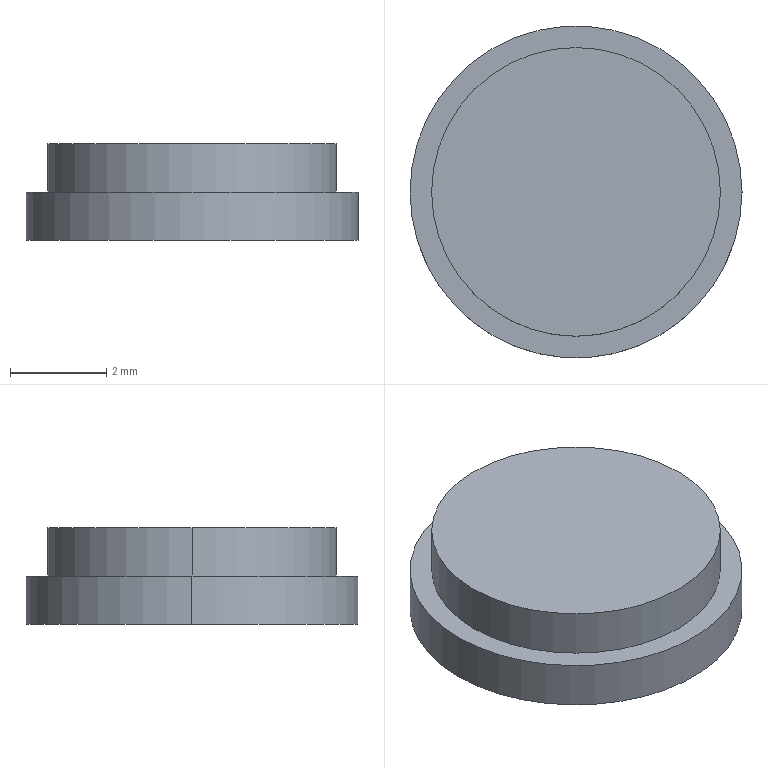Part | SolidWorks | features Extrusion 1, ICE 1 | 1 solid | 7 faces | box 6.9 x 6.9 x 2 mm | volume 65.667 mm3 | cylinder 4 | plane 3 | commonest cylinder face diameters 6 x2 6.9 x2
STEP:
#1=CARTESIAN_POINT('',(3.45,0.,-1.));
#2=VERTEX_POINT('',#1);
#3=CARTESIAN_POINT('',(-3.45,0.,-1.));
#4=VERTEX_POINT('',#3);
#5=CARTESIAN_POINT('',(0.,0.,-1.));
#6=DIRECTION('',(0.,0.,1.));
#7=DIRECTION('',(1.,0.,0.));
#8=AXIS2_PLACEMENT_3D('',#5,#6,#7);
#9=CIRCLE('',#8,3.45);
#10=EDGE_CURVE('',#2,#4,#9,.T.);
#11=ORIENTED_EDGE('',*,*,#10,.T.);
#12=CARTESIAN_POINT('',(-3.45,0.,0.));
#13=VERTEX_POINT('',#12);
#14=CARTESIAN_POINT('',(-3.45,0.,-1.));
#15=DIRECTION('',(0.,0.,1.));
#16=VECTOR('',#15,1000.);
#17=LINE('',#14,#16);
#18=EDGE_CURVE('',#4,#13,#17,.T.);
#19=ORIENTED_EDGE('',*,*,#18,.T.);
#20=CARTESIAN_POINT('',(3.45,0.,0.));
#21=VERTEX_POINT('',#20);
#22=CARTESIAN_POINT('',(0.,0.,0.));
#23=DIRECTION('',(0.,0.,1.));
#24=DIRECTION('',(1.,0.,0.));
#25=AXIS2_PLACEMENT_3D('',#22,#23,#24);
#26=CIRCLE('',#25,3.45);
#27=EDGE_CURVE('',#21,#13,#26,.T.);
#28=ORIENTED_EDGE('',*,*,#27,.F.);
#29=CARTESIAN_POINT('',(3.45,0.,-1.));
#30=DIRECTION('',(0.,0.,1.));
#31=VECTOR('',#30,1000.);
#32=LINE('',#29,#31);
#33=EDGE_CURVE('',#2,#21,#32,.T.);
#34=ORIENTED_EDGE('',*,*,#33,.F.);
#35=EDGE_LOOP('',(#11,#19,#28,#34));
#36=FACE_OUTER_BOUND('',#35,.T.);
#37=CARTESIAN_POINT('',(0.,0.,-1.));
#38=DIRECTION('',(0.,0.,1.));
#39=DIRECTION('',(1.,0.,0.));
#40=AXIS2_PLACEMENT_3D('',#37,#38,#39);
#41=CYLINDRICAL_SURFACE('',#40,3.45);
#42=ADVANCED_FACE('',(#36),#41,.T.);
#43=CARTESIAN_POINT('',(3.,0.,1.));
#44=VERTEX_POINT('',#43);
#45=CARTESIAN_POINT('',(-3.,0.,1.));
#46=VERTEX_POINT('',#45);
#47=CARTESIAN_POINT('',(0.,0.,1.));
#48=DIRECTION('',(0.,0.,1.));
#49=DIRECTION('',(1.,0.,0.));
#50=AXIS2_PLACEMENT_3D('',#47,#48,#49);
#51=CIRCLE('',#50,3.);
#52=EDGE_CURVE('',#44,#46,#51,.T.);
#53=ORIENTED_EDGE('',*,*,#52,.F.);
#54=CARTESIAN_POINT('',(3.,0.,0.));
#55=VERTEX_POINT('',#54);
#56=CARTESIAN_POINT('',(3.,0.,1.));
#57=DIRECTION('',(0.,0.,-1.));
#58=VECTOR('',#57,1000.);
#59=LINE('',#56,#58);
#60=EDGE_CURVE('',#44,#55,#59,.T.);
#61=ORIENTED_EDGE('',*,*,#60,.T.);
#62=CARTESIAN_POINT('',(-3.,0.,0.));
#63=VERTEX_POINT('',#62);
#64=CARTESIAN_POINT('',(0.,0.,0.));
#65=DIRECTION('',(0.,0.,1.));
#66=DIRECTION('',(1.,0.,0.));
#67=AXIS2_PLACEMENT_3D('',#64,#65,#66);
#68=CIRCLE('',#67,3.);
#69=EDGE_CURVE('',#55,#63,#68,.T.);
#70=ORIENTED_EDGE('',*,*,#69,.T.);
#71=CARTESIAN_POINT('',(-3.,0.,1.));
#72=DIRECTION('',(0.,0.,-1.));
#73=VECTOR('',#72,1000.);
#74=LINE('',#71,#73);
#75=EDGE_CURVE('',#46,#63,#74,.T.);
#76=ORIENTED_EDGE('',*,*,#75,.F.);
#77=EDGE_LOOP('',(#53,#61,#70,#76));
#78=FACE_OUTER_BOUND('',#77,.T.);
#79=CARTESIAN_POINT('',(0.,0.,1.));
#80=DIRECTION('',(0.,0.,-1.));
#81=DIRECTION('',(-1.,0.,0.));
#82=AXIS2_PLACEMENT_3D('',#79,#80,#81);
#83=CYLINDRICAL_SURFACE('',#82,3.);
#84=ADVANCED_FACE('',(#78),#83,.T.);
#85=ORIENTED_EDGE('',*,*,#60,.F.);
#86=CARTESIAN_POINT('',(0.,0.,1.));
#87=DIRECTION('',(0.,0.,1.));
#88=DIRECTION('',(1.,0.,0.));
#89=AXIS2_PLACEMENT_3D('',#86,#87,#88);
#90=CIRCLE('',#89,3.);
#91=EDGE_CURVE('',#46,#44,#90,.T.);
#92=ORIENTED_EDGE('',*,*,#91,.F.);
#93=ORIENTED_EDGE('',*,*,#75,.T.);
#94=CARTESIAN_POINT('',(0.,0.,0.));
#95=DIRECTION('',(0.,0.,1.));
#96=DIRECTION('',(1.,0.,0.));
#97=AXIS2_PLACEMENT_3D('',#94,#95,#96);
#98=CIRCLE('',#97,3.);
#99=EDGE_CURVE('',#63,#55,#98,.T.);
#100=ORIENTED_EDGE('',*,*,#99,.T.);
#101=EDGE_LOOP('',(#85,#92,#93,#100));
#102=FACE_OUTER_BOUND('',#101,.T.);
#103=CARTESIAN_POINT('',(0.,0.,1.));
#104=DIRECTION('',(0.,0.,-1.));
#105=DIRECTION('',(-1.,0.,0.));
#106=AXIS2_PLACEMENT_3D('',#103,#104,#105);
#107=CYLINDRICAL_SURFACE('',#106,3.);
#108=ADVANCED_FACE('',(#102),#107,.T.);
#109=ORIENTED_EDGE('',*,*,#91,.T.);
#110=ORIENTED_EDGE('',*,*,#52,.T.);
#111=EDGE_LOOP('',(#109,#110));
#112=FACE_OUTER_BOUND('',#111,.T.);
#113=CARTESIAN_POINT('',(0.,0.,1.));
#114=DIRECTION('',(0.,0.,1.));
#115=DIRECTION('',(1.,0.,0.));
#116=AXIS2_PLACEMENT_3D('',#113,#114,#115);
#117=PLANE('',#116);
#118=ADVANCED_FACE('',(#112),#117,.T.);
#119=ORIENTED_EDGE('',*,*,#18,.F.);
#120=CARTESIAN_POINT('',(0.,0.,-1.));
#121=DIRECTION('',(0.,0.,1.));
#122=DIRECTION('',(1.,0.,0.));
#123=AXIS2_PLACEMENT_3D('',#120,#121,#122);
#124=CIRCLE('',#123,3.45);
#125=EDGE_CURVE('',#4,#2,#124,.T.);
#126=ORIENTED_EDGE('',*,*,#125,.T.);
#127=ORIENTED_EDGE('',*,*,#33,.T.);
#128=CARTESIAN_POINT('',(0.,0.,0.));
#129=DIRECTION('',(0.,0.,1.));
#130=DIRECTION('',(1.,0.,0.));
#131=AXIS2_PLACEMENT_3D('',#128,#129,#130);
#132=CIRCLE('',#131,3.45);
#133=EDGE_CURVE('',#13,#21,#132,.T.);
#134=ORIENTED_EDGE('',*,*,#133,.F.);
#135=EDGE_LOOP('',(#119,#126,#127,#134));
#136=FACE_OUTER_BOUND('',#135,.T.);
#137=CARTESIAN_POINT('',(0.,0.,-1.));
#138=DIRECTION('',(0.,0.,1.));
#139=DIRECTION('',(1.,0.,0.));
#140=AXIS2_PLACEMENT_3D('',#137,#138,#139);
#141=CYLINDRICAL_SURFACE('',#140,3.45);
#142=ADVANCED_FACE('',(#136),#141,.T.);
#143=ORIENTED_EDGE('',*,*,#10,.F.);
#144=ORIENTED_EDGE('',*,*,#125,.F.);
#145=EDGE_LOOP('',(#143,#144));
#146=FACE_OUTER_BOUND('',#145,.T.);
#147=CARTESIAN_POINT('',(0.,0.,-1.));
#148=DIRECTION('',(0.,0.,1.));
#149=DIRECTION('',(1.,0.,0.));
#150=AXIS2_PLACEMENT_3D('',#147,#148,#149);
#151=PLANE('',#150);
#152=ADVANCED_FACE('',(#146),#151,.F.);
#153=ORIENTED_EDGE('',*,*,#99,.F.);
#154=ORIENTED_EDGE('',*,*,#69,.F.);
#155=EDGE_LOOP('',(#153,#154));
#156=FACE_BOUND('',#155,.T.);
#157=ORIENTED_EDGE('',*,*,#27,.T.);
#158=ORIENTED_EDGE('',*,*,#133,.T.);
#159=EDGE_LOOP('',(#157,#158));
#160=FACE_OUTER_BOUND('',#159,.T.);
#161=CARTESIAN_POINT('',(0.,0.,0.));
#162=DIRECTION('',(0.,0.,1.));
#163=DIRECTION('',(1.,0.,0.));
#164=AXIS2_PLACEMENT_3D('',#161,#162,#163);
#165=PLANE('',#164);
#166=ADVANCED_FACE('',(#156,#160),#165,.T.);
#167=CLOSED_SHELL('',(#42,#84,#108,#118,#142,#152,#166));
#168=MANIFOLD_SOLID_BREP('',#167);
#169=CARTESIAN_POINT('',(0.,0.,0.));
#170=DIRECTION('',(0.,0.,1.));
#171=DIRECTION('',(1.,0.,0.));
#172=AXIS2_PLACEMENT_3D('',#169,#170,#171);
#173=(LENGTH_UNIT()NAMED_UNIT(*)SI_UNIT(.MILLI.,.METRE.));
#174=UNCERTAINTY_MEASURE_WITH_UNIT(LENGTH_MEASURE(0.00001),#173,'','');
#175=(NAMED_UNIT(*)PLANE_ANGLE_UNIT()SI_UNIT($,.RADIAN.));
#176=(NAMED_UNIT(*)SI_UNIT($,.STERADIAN.)SOLID_ANGLE_UNIT());
#177=(GEOMETRIC_REPRESENTATION_CONTEXT(3)GLOBAL_UNCERTAINTY_ASSIGNED_CONTEXT((#174))GLOBAL_UNIT_ASSIGNED_CONTEXT((#173,#175,#176))REPRESENTATION_CONTEXT('',''));
#178=ADVANCED_BREP_SHAPE_REPRESENTATION('',(#168,#172),#177);